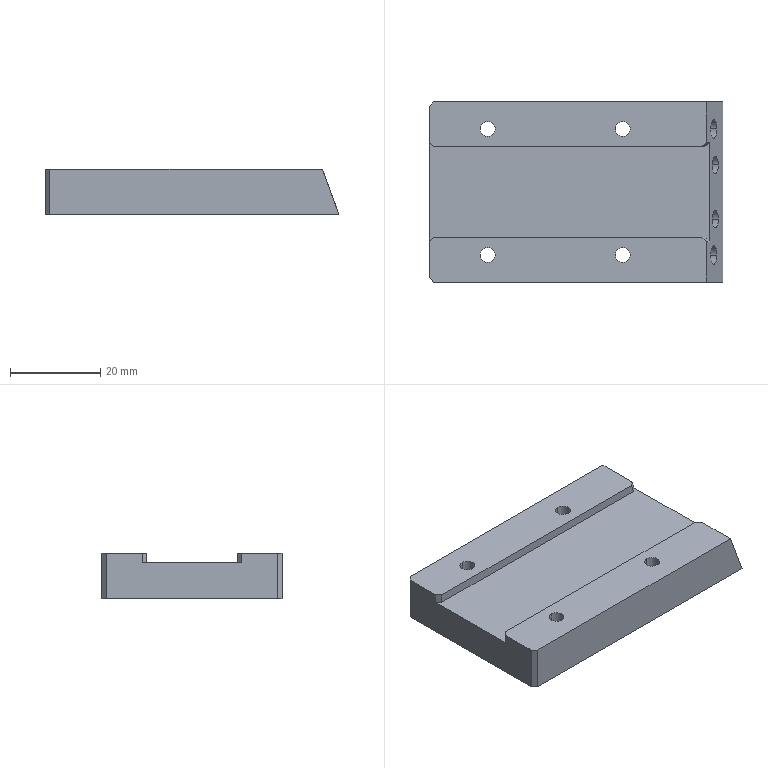NC program | NX | posted with a generic post | part box 65.2 x 40 x 10 mm
Whole program:
N10 G17 G21 G94 G90
(FLOOR_WALL_COPY_COPY , TOOL : D50R0.8)
N12 T03 M6
N14 G54
N16 G17 G0 G90 X-93.2 Y0. S1000 M3
N18 G43 Z30. H3
N20 Z7.715
N22 G94 G1 Z4.715 F1500.
N24 X-90.2
N26 X25.
N28 X28.
N30 Z7.715
N32 G0 Z30.
N34 X-93.2
N36 Z7.429
N38 G1 Z4.429
N40 X-90.2
N42 X25.
N44 X28.
N46 Z7.429
N48 G0 Z30.
N50 X-93.2
N52 Z7.144
N54 G1 Z4.144
N56 X-90.2
N58 X25.
N60 X28.
N62 Z7.144
N64 G0 Z30.
N66 X-93.2
N68 Z6.859
N70 G1 Z3.859
N72 X-90.2
N74 X25.
N76 X28.
N78 Z6.859
N80 G0 Z30.
N82 X-93.2
N84 Z6.573
N86 G1 Z3.573
N88 X-90.2
N90 X25.
N92 X28.
N94 Z6.573
N96 G0 Z30.
N98 X-93.2
N100 Z6.288
N102 G1 Z3.288
N104 X-90.2
N106 X25.
N108 X28.
N110 Z6.288
N112 G0 Z30.
N114 X-93.2
N116 Z6.003
N118 G1 Z3.003
N120 X-90.2
N122 X25.
N124 X28.
N126 Z6.003
N128 G0 Z30.
N130 X-93.2
N132 Z5.718
N134 G1 Z2.718
N136 X-90.2
N138 X25.
N140 X28.
N142 Z5.718
N144 G0 Z30.
N146 X-93.2
N148 Z5.432
N150 G1 Z2.432
N152 X-90.2
N154 X25.
N156 X28.
N158 Z5.432
N160 G0 Z30.
N162 X-93.2
N164 Z5.147
N166 G1 Z2.147
N168 X-90.2
N170 X25.
N172 X28.
N174 Z5.147
N176 G0 Z30.
N178 X-93.2
N180 Z4.862
N182 G1 Z1.862
N184 X-90.2
N186 X25.
N188 X28.
N190 Z4.862
N192 G0 Z30.
N194 X-93.2
N196 Z4.576
N198 G1 Z1.576
N200 X-90.2
N202 X25.
N204 X28.
N206 Z4.576
N208 G0 Z30.
N210 X-93.2
N212 Z4.291
N214 G1 Z1.291
N216 X-90.2
N218 X25.
N220 X28.
N222 Z4.291
N224 G0 Z30.
N226 X-93.2
N228 Z4.006
N230 G1 Z1.006
N232 X-90.2
N234 X25.
N236 X28.
N238 Z4.006
N240 G0 Z30.
N242 X-93.2
N244 Z3.721
N246 G1 Z0.721
N248 X-90.2
N250 X25.
N252 X28.
N254 Z3.721
N256 G0 Z30.
N258 X-93.2
N260 Z3.435
N262 G1 Z0.435
N264 X-90.2
N266 X25.
N268 X28.
N270 Z3.435
N272 G0 Z30.
N274 X-93.2
N276 Z3.15
N278 G1 Z0.15
N280 X-90.2
N282 X25.
N284 X28.
N286 Z3.15
N288 G0 Z30.
(11_COPY_COPY_COPY_COPY_COPY_1 , TOOL : D6A45)
N290 T01 M6
N292 G17 G43 G0 G90 X-43. Y14.691 Z30. S7500 H1 M3
N294 Z3.
N296 G94 G1 Z-1. F1000.
N298 X-43.004
N300 G3 X-43.691 Y13.996 R0.691
N302 X-43. Y14.691 R-0.691
N304 X-43.52 Y14.391 R0.6
N306 G1 Z2.
N308 G0 Z30.
N310 X-13. Y-14.691
N312 Z3.
N314 G1 Z-1.
N316 G3 X-12.309 Y-14. R0.691
N318 X-13. Y-14.691 R-0.691
N320 X-12.48 Y-14.391 R0.6
N322 G1 Z2.
N324 G0 Z30.
N326 X-43. Y-14.691
N328 Z3.
N330 G1 Z-1.
N332 G3 X-42.309 Y-14. R0.691
N334 X-43. Y-14.691 R-0.691
N336 X-42.48 Y-14.391 R0.6
N338 G1 Z2.
N340 G0 Z30.
N342 X-13. Y14.691
N344 Z3.
N346 G1 Z-1.
N348 X-13.004
N350 G3 X-13.691 Y13.996 R0.691
N352 X-13. Y14.691 R-0.691
N354 X-13.52 Y14.391 R0.6
N356 G1 Z2.
N358 G0 Z30.
N360 X-66.121 Y21.952
N362 Z2.
N364 G1 Z-1.
N366 X-65.721 Y21.259
N368 G3 X-65.201 Y20.959 R0.6
N370 G1 X-0.999
N372 G2 X-0.323 Y20.678 R0.957
N374 G1 X0.678 Y19.677
N376 G2 X0.959 Y19.001 R0.956
N378 G1 Y-19.001
N380 G2 X0.678 Y-19.677 R0.956
N382 G1 X-0.323 Y-20.678
N384 G2 X-0.999 Y-20.959 R0.957
N386 G1 X-65.201
N388 G2 X-66.159 Y-20.001 R0.958
N390 G1 Y20.001
N392 G2 X-65.201 Y20.959 R0.958
N394 G3 X-64.681 Y21.259 R0.6
N396 G1 X-64.162 Y22.159
N398 Z2.
N400 G0 Z30.
N402 M5
N404 M2